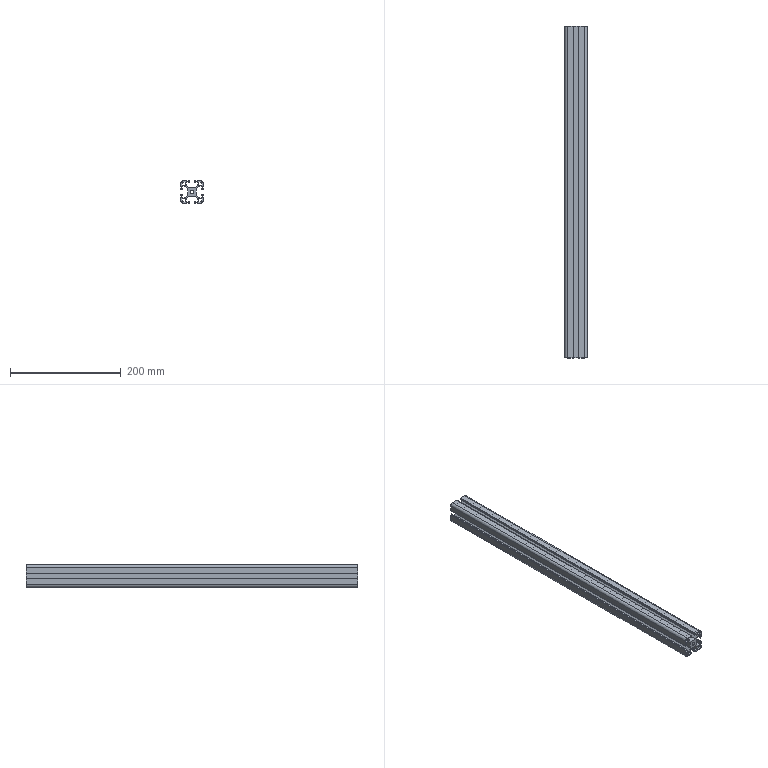Part | 1 solid | 104 faces | box 40 x 600 x 40 mm | volume 345927 mm3 | plane 94 | cylinder 10 | commonest cylinder face diameters 5 x4 9 x4 6.8 x2